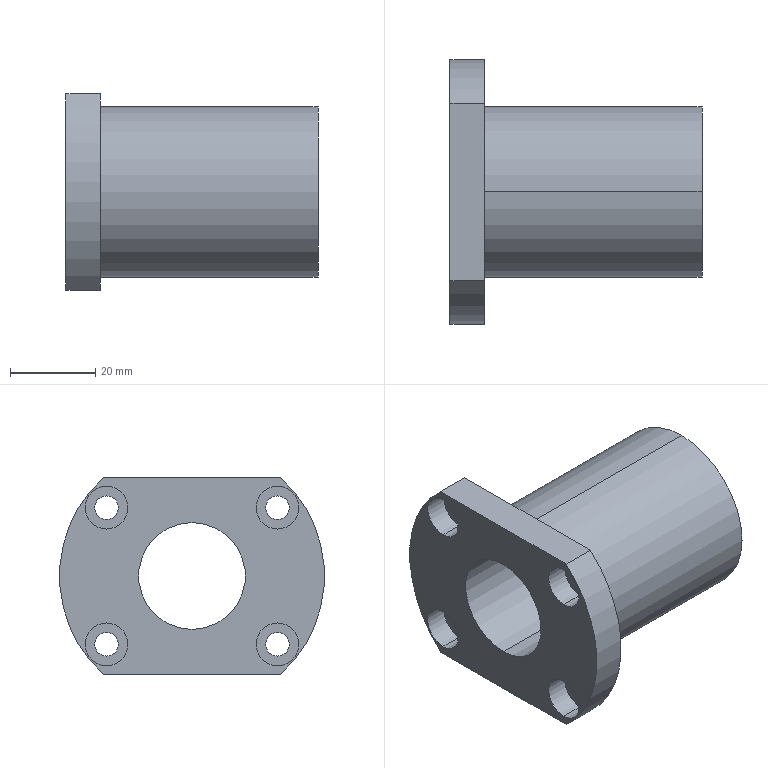Part | STEP file | Linear bearing LMH25UU | 1 solid | 31 faces | box 59 x 62 x 46 mm | volume 53686 mm3 | cylinder 22 | plane 9 | commonest cylinder face diameters 5.5 x8 10 x8 25 x2 40 x2 62 x2